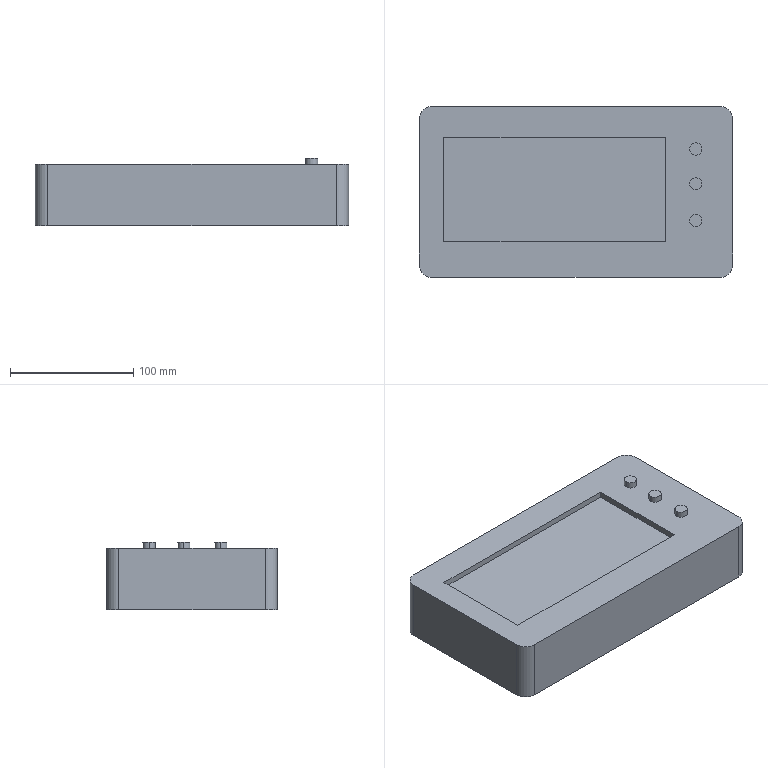Part | STEP file | Controller | 1 solid | 27 faces | box 254.791 x 138.794 x 55 mm | volume 1688527 mm3 | plane 15 | cylinder 12 | commonest cylinder face diameters 10 x6 20 x4 2 x2
STEP:
#1=CARTESIAN_POINT('',(-10.,-56.504,29.99));
#2=VERTEX_POINT('',#1);
#3=CARTESIAN_POINT('',(-10.,-56.504,27.99));
#4=VERTEX_POINT('',#3);
#5=CARTESIAN_POINT('',(-10.,-56.504,28.99));
#6=DIRECTION('',(1.,0.,0.));
#7=DIRECTION('',(0.,0.,-1.));
#8=AXIS2_PLACEMENT_3D('',#5,#6,#7);
#9=CIRCLE('',#8,1.);
#10=EDGE_CURVE('',#2,#4,#9,.T.);
#11=ORIENTED_EDGE('',*,*,#10,.F.);
#12=CARTESIAN_POINT('',(0.,-56.504,29.99));
#13=VERTEX_POINT('',#12);
#14=CARTESIAN_POINT('',(-10.,-56.504,29.99));
#15=DIRECTION('',(1.,0.,0.));
#16=VECTOR('',#15,1000.);
#17=LINE('',#14,#16);
#18=EDGE_CURVE('',#2,#13,#17,.T.);
#19=ORIENTED_EDGE('',*,*,#18,.T.);
#20=CARTESIAN_POINT('',(0.,-56.504,27.99));
#21=VERTEX_POINT('',#20);
#22=CARTESIAN_POINT('',(0.,-56.504,28.99));
#23=DIRECTION('',(1.,0.,0.));
#24=DIRECTION('',(0.,0.,-1.));
#25=AXIS2_PLACEMENT_3D('',#22,#23,#24);
#26=CIRCLE('',#25,1.);
#27=EDGE_CURVE('',#13,#21,#26,.T.);
#28=ORIENTED_EDGE('',*,*,#27,.T.);
#29=CARTESIAN_POINT('',(-10.,-56.504,27.99));
#30=DIRECTION('',(1.,0.,0.));
#31=VECTOR('',#30,1000.);
#32=LINE('',#29,#31);
#33=EDGE_CURVE('',#4,#21,#32,.T.);
#34=ORIENTED_EDGE('',*,*,#33,.F.);
#35=EDGE_LOOP('',(#11,#19,#28,#34));
#36=FACE_OUTER_BOUND('',#35,.T.);
#37=CARTESIAN_POINT('',(-10.,-56.504,28.99));
#38=DIRECTION('',(1.,0.,0.));
#39=DIRECTION('',(0.,0.,-1.));
#40=AXIS2_PLACEMENT_3D('',#37,#38,#39);
#41=CYLINDRICAL_SURFACE('',#40,1.);
#42=ADVANCED_FACE('',(#36),#41,.F.);
#43=CARTESIAN_POINT('',(-25.,-92.807,55.));
#44=VERTEX_POINT('',#43);
#45=CARTESIAN_POINT('',(-35.,-92.807,55.));
#46=VERTEX_POINT('',#45);
#47=CARTESIAN_POINT('',(-30.,-92.807,55.));
#48=DIRECTION('',(0.,0.,1.));
#49=DIRECTION('',(1.,0.,0.));
#50=AXIS2_PLACEMENT_3D('',#47,#48,#49);
#51=CIRCLE('',#50,5.);
#52=EDGE_CURVE('',#44,#46,#51,.T.);
#53=ORIENTED_EDGE('',*,*,#52,.F.);
#54=CARTESIAN_POINT('',(-25.,-92.807,50.));
#55=VERTEX_POINT('',#54);
#56=CARTESIAN_POINT('',(-25.,-92.807,55.));
#57=DIRECTION('',(0.,0.,-1.));
#58=VECTOR('',#57,1000.);
#59=LINE('',#56,#58);
#60=EDGE_CURVE('',#44,#55,#59,.T.);
#61=ORIENTED_EDGE('',*,*,#60,.T.);
#62=CARTESIAN_POINT('',(-35.,-92.807,50.));
#63=VERTEX_POINT('',#62);
#64=CARTESIAN_POINT('',(-30.,-92.807,50.));
#65=DIRECTION('',(0.,0.,1.));
#66=DIRECTION('',(1.,0.,0.));
#67=AXIS2_PLACEMENT_3D('',#64,#65,#66);
#68=CIRCLE('',#67,5.);
#69=EDGE_CURVE('',#55,#63,#68,.T.);
#70=ORIENTED_EDGE('',*,*,#69,.T.);
#71=CARTESIAN_POINT('',(-35.,-92.807,55.));
#72=DIRECTION('',(0.,0.,-1.));
#73=VECTOR('',#72,1000.);
#74=LINE('',#71,#73);
#75=EDGE_CURVE('',#46,#63,#74,.T.);
#76=ORIENTED_EDGE('',*,*,#75,.F.);
#77=EDGE_LOOP('',(#53,#61,#70,#76));
#78=FACE_OUTER_BOUND('',#77,.T.);
#79=CARTESIAN_POINT('',(-30.,-92.807,55.));
#80=DIRECTION('',(0.,0.,-1.));
#81=DIRECTION('',(-1.,0.,0.));
#82=AXIS2_PLACEMENT_3D('',#79,#80,#81);
#83=CYLINDRICAL_SURFACE('',#82,5.);
#84=ADVANCED_FACE('',(#78),#83,.T.);
#85=CARTESIAN_POINT('',(-25.,-62.807,55.));
#86=VERTEX_POINT('',#85);
#87=CARTESIAN_POINT('',(-35.,-62.807,55.));
#88=VERTEX_POINT('',#87);
#89=CARTESIAN_POINT('',(-30.,-62.807,55.));
#90=DIRECTION('',(0.,0.,1.));
#91=DIRECTION('',(1.,0.,0.));
#92=AXIS2_PLACEMENT_3D('',#89,#90,#91);
#93=CIRCLE('',#92,5.);
#94=EDGE_CURVE('',#86,#88,#93,.T.);
#95=ORIENTED_EDGE('',*,*,#94,.F.);
#96=CARTESIAN_POINT('',(-25.,-62.807,50.));
#97=VERTEX_POINT('',#96);
#98=CARTESIAN_POINT('',(-25.,-62.807,55.));
#99=DIRECTION('',(0.,0.,-1.));
#100=VECTOR('',#99,1000.);
#101=LINE('',#98,#100);
#102=EDGE_CURVE('',#86,#97,#101,.T.);
#103=ORIENTED_EDGE('',*,*,#102,.T.);
#104=CARTESIAN_POINT('',(-35.,-62.807,50.));
#105=VERTEX_POINT('',#104);
#106=CARTESIAN_POINT('',(-30.,-62.807,50.));
#107=DIRECTION('',(0.,0.,1.));
#108=DIRECTION('',(1.,0.,0.));
#109=AXIS2_PLACEMENT_3D('',#106,#107,#108);
#110=CIRCLE('',#109,5.);
#111=EDGE_CURVE('',#97,#105,#110,.T.);
#112=ORIENTED_EDGE('',*,*,#111,.T.);
#113=CARTESIAN_POINT('',(-35.,-62.807,55.));
#114=DIRECTION('',(0.,0.,-1.));
#115=VECTOR('',#114,1000.);
#116=LINE('',#113,#115);
#117=EDGE_CURVE('',#88,#105,#116,.T.);
#118=ORIENTED_EDGE('',*,*,#117,.F.);
#119=EDGE_LOOP('',(#95,#103,#112,#118));
#120=FACE_OUTER_BOUND('',#119,.T.);
#121=CARTESIAN_POINT('',(-30.,-62.807,55.));
#122=DIRECTION('',(0.,0.,-1.));
#123=DIRECTION('',(-1.,0.,0.));
#124=AXIS2_PLACEMENT_3D('',#121,#122,#123);
#125=CYLINDRICAL_SURFACE('',#124,5.);
#126=ADVANCED_FACE('',(#120),#125,.T.);
#127=CARTESIAN_POINT('',(-25.,-34.514,55.));
#128=VERTEX_POINT('',#127);
#129=CARTESIAN_POINT('',(-35.,-34.514,55.));
#130=VERTEX_POINT('',#129);
#131=CARTESIAN_POINT('',(-30.,-34.514,55.));
#132=DIRECTION('',(0.,0.,1.));
#133=DIRECTION('',(1.,0.,0.));
#134=AXIS2_PLACEMENT_3D('',#131,#132,#133);
#135=CIRCLE('',#134,5.);
#136=EDGE_CURVE('',#128,#130,#135,.T.);
#137=ORIENTED_EDGE('',*,*,#136,.F.);
#138=CARTESIAN_POINT('',(-25.,-34.514,50.));
#139=VERTEX_POINT('',#138);
#140=CARTESIAN_POINT('',(-25.,-34.514,55.));
#141=DIRECTION('',(0.,0.,-1.));
#142=VECTOR('',#141,1000.);
#143=LINE('',#140,#142);
#144=EDGE_CURVE('',#128,#139,#143,.T.);
#145=ORIENTED_EDGE('',*,*,#144,.T.);
#146=CARTESIAN_POINT('',(-35.,-34.514,50.));
#147=VERTEX_POINT('',#146);
#148=CARTESIAN_POINT('',(-30.,-34.514,50.));
#149=DIRECTION('',(0.,0.,1.));
#150=DIRECTION('',(1.,0.,0.));
#151=AXIS2_PLACEMENT_3D('',#148,#149,#150);
#152=CIRCLE('',#151,5.);
#153=EDGE_CURVE('',#139,#147,#152,.T.);
#154=ORIENTED_EDGE('',*,*,#153,.T.);
#155=CARTESIAN_POINT('',(-35.,-34.514,55.));
#156=DIRECTION('',(0.,0.,-1.));
#157=VECTOR('',#156,1000.);
#158=LINE('',#155,#157);
#159=EDGE_CURVE('',#130,#147,#158,.T.);
#160=ORIENTED_EDGE('',*,*,#159,.F.);
#161=EDGE_LOOP('',(#137,#145,#154,#160));
#162=FACE_OUTER_BOUND('',#161,.T.);
#163=CARTESIAN_POINT('',(-30.,-34.514,55.));
#164=DIRECTION('',(0.,0.,-1.));
#165=DIRECTION('',(-1.,0.,0.));
#166=AXIS2_PLACEMENT_3D('',#163,#164,#165);
#167=CYLINDRICAL_SURFACE('',#166,5.);
#168=ADVANCED_FACE('',(#162),#167,.T.);
#169=CARTESIAN_POINT('',(-254.791,-128.794,0.));
#170=VERTEX_POINT('',#169);
#171=CARTESIAN_POINT('',(-244.791,-138.794,0.));
#172=VERTEX_POINT('',#171);
#173=CARTESIAN_POINT('',(-244.791,-128.794,0.));
#174=DIRECTION('',(0.,0.,1.));
#175=DIRECTION('',(1.,0.,0.));
#176=AXIS2_PLACEMENT_3D('',#173,#174,#175);
#177=CIRCLE('',#176,10.);
#178=EDGE_CURVE('',#170,#172,#177,.T.);
#179=ORIENTED_EDGE('',*,*,#178,.T.);
#180=CARTESIAN_POINT('',(-244.791,-138.794,50.));
#181=VERTEX_POINT('',#180);
#182=CARTESIAN_POINT('',(-244.791,-138.794,50.));
#183=DIRECTION('',(0.,0.,-1.));
#184=VECTOR('',#183,1000.);
#185=LINE('',#182,#184);
#186=EDGE_CURVE('',#181,#172,#185,.T.);
#187=ORIENTED_EDGE('',*,*,#186,.F.);
#188=CARTESIAN_POINT('',(-254.791,-128.794,50.));
#189=VERTEX_POINT('',#188);
#190=CARTESIAN_POINT('',(-244.791,-128.794,50.));
#191=DIRECTION('',(0.,0.,1.));
#192=DIRECTION('',(1.,0.,0.));
#193=AXIS2_PLACEMENT_3D('',#190,#191,#192);
#194=CIRCLE('',#193,10.);
#195=EDGE_CURVE('',#189,#181,#194,.T.);
#196=ORIENTED_EDGE('',*,*,#195,.F.);
#197=CARTESIAN_POINT('',(-254.791,-128.794,50.));
#198=DIRECTION('',(0.,0.,-1.));
#199=VECTOR('',#198,1000.);
#200=LINE('',#197,#199);
#201=EDGE_CURVE('',#189,#170,#200,.T.);
#202=ORIENTED_EDGE('',*,*,#201,.T.);
#203=EDGE_LOOP('',(#179,#187,#196,#202));
#204=FACE_OUTER_BOUND('',#203,.T.);
#205=CARTESIAN_POINT('',(-244.791,-128.794,50.));
#206=DIRECTION('',(0.,0.,-1.));
#207=DIRECTION('',(-1.,0.,0.));
#208=AXIS2_PLACEMENT_3D('',#205,#206,#207);
#209=CYLINDRICAL_SURFACE('',#208,10.);
#210=ADVANCED_FACE('',(#204),#209,.T.);
#211=CARTESIAN_POINT('',(-10.,-138.794,0.));
#212=VERTEX_POINT('',#211);
#213=CARTESIAN_POINT('',(-244.791,-138.794,0.));
#214=DIRECTION('',(1.,0.,0.));
#215=VECTOR('',#214,1000.);
#216=LINE('',#213,#215);
#217=EDGE_CURVE('',#172,#212,#216,.T.);
#218=ORIENTED_EDGE('',*,*,#217,.T.);
#219=CARTESIAN_POINT('',(-10.,-138.794,50.));
#220=VERTEX_POINT('',#219);
#221=CARTESIAN_POINT('',(-10.,-138.794,50.));
#222=DIRECTION('',(0.,0.,-1.));
#223=VECTOR('',#222,1000.);
#224=LINE('',#221,#223);
#225=EDGE_CURVE('',#220,#212,#224,.T.);
#226=ORIENTED_EDGE('',*,*,#225,.F.);
#227=CARTESIAN_POINT('',(-244.791,-138.794,50.));
#228=DIRECTION('',(1.,0.,0.));
#229=VECTOR('',#228,1000.);
#230=LINE('',#227,#229);
#231=EDGE_CURVE('',#181,#220,#230,.T.);
#232=ORIENTED_EDGE('',*,*,#231,.F.);
#233=ORIENTED_EDGE('',*,*,#186,.T.);
#234=EDGE_LOOP('',(#218,#226,#232,#233));
#235=FACE_OUTER_BOUND('',#234,.T.);
#236=CARTESIAN_POINT('',(-244.791,-138.794,50.));
#237=DIRECTION('',(0.,1.,0.));
#238=DIRECTION('',(0.,0.,1.));
#239=AXIS2_PLACEMENT_3D('',#236,#237,#238);
#240=PLANE('',#239);
#241=ADVANCED_FACE('',(#235),#240,.F.);
#242=CARTESIAN_POINT('',(0.,-128.794,0.));
#243=VERTEX_POINT('',#242);
#244=CARTESIAN_POINT('',(-10.,-128.794,0.));
#245=DIRECTION('',(0.,0.,1.));
#246=DIRECTION('',(1.,0.,0.));
#247=AXIS2_PLACEMENT_3D('',#244,#245,#246);
#248=CIRCLE('',#247,10.);
#249=EDGE_CURVE('',#212,#243,#248,.T.);
#250=ORIENTED_EDGE('',*,*,#249,.T.);
#251=CARTESIAN_POINT('',(0.,-128.794,50.));
#252=VERTEX_POINT('',#251);
#253=CARTESIAN_POINT('',(0.,-128.794,50.));
#254=DIRECTION('',(0.,0.,-1.));
#255=VECTOR('',#254,1000.);
#256=LINE('',#253,#255);
#257=EDGE_CURVE('',#252,#243,#256,.T.);
#258=ORIENTED_EDGE('',*,*,#257,.F.);
#259=CARTESIAN_POINT('',(-10.,-128.794,50.));
#260=DIRECTION('',(0.,0.,1.));
#261=DIRECTION('',(1.,0.,0.));
#262=AXIS2_PLACEMENT_3D('',#259,#260,#261);
#263=CIRCLE('',#262,10.);
#264=EDGE_CURVE('',#220,#252,#263,.T.);
#265=ORIENTED_EDGE('',*,*,#264,.F.);
#266=ORIENTED_EDGE('',*,*,#225,.T.);
#267=EDGE_LOOP('',(#250,#258,#265,#266));
#268=FACE_OUTER_BOUND('',#267,.T.);
#269=CARTESIAN_POINT('',(-10.,-128.794,50.));
#270=DIRECTION('',(0.,0.,-1.));
#271=DIRECTION('',(-1.,0.,0.));
#272=AXIS2_PLACEMENT_3D('',#269,#270,#271);
#273=CYLINDRICAL_SURFACE('',#272,10.);
#274=ADVANCED_FACE('',(#268),#273,.T.);
#275=CARTESIAN_POINT('',(0.,-56.504,28.99));
#276=DIRECTION('',(1.,0.,0.));
#277=DIRECTION('',(0.,0.,-1.));
#278=AXIS2_PLACEMENT_3D('',#275,#276,#277);
#279=CIRCLE('',#278,1.);
#280=EDGE_CURVE('',#21,#13,#279,.T.);
#281=ORIENTED_EDGE('',*,*,#280,.F.);
#282=ORIENTED_EDGE('',*,*,#27,.F.);
#283=EDGE_LOOP('',(#281,#282));
#284=FACE_BOUND('',#283,.T.);
#285=CARTESIAN_POINT('',(0.,-10.,0.));
#286=VERTEX_POINT('',#285);
#287=CARTESIAN_POINT('',(0.,-128.794,0.));
#288=DIRECTION('',(0.,1.,0.));
#289=VECTOR('',#288,1000.);
#290=LINE('',#287,#289);
#291=EDGE_CURVE('',#243,#286,#290,.T.);
#292=ORIENTED_EDGE('',*,*,#291,.T.);
#293=CARTESIAN_POINT('',(0.,-10.,50.));
#294=VERTEX_POINT('',#293);
#295=CARTESIAN_POINT('',(0.,-10.,50.));
#296=DIRECTION('',(0.,0.,-1.));
#297=VECTOR('',#296,1000.);
#298=LINE('',#295,#297);
#299=EDGE_CURVE('',#294,#286,#298,.T.);
#300=ORIENTED_EDGE('',*,*,#299,.F.);
#301=CARTESIAN_POINT('',(0.,-128.794,50.));
#302=DIRECTION('',(0.,1.,0.));
#303=VECTOR('',#302,1000.);
#304=LINE('',#301,#303);
#305=EDGE_CURVE('',#252,#294,#304,.T.);
#306=ORIENTED_EDGE('',*,*,#305,.F.);
#307=ORIENTED_EDGE('',*,*,#257,.T.);
#308=EDGE_LOOP('',(#292,#300,#306,#307));
#309=FACE_OUTER_BOUND('',#308,.T.);
#310=CARTESIAN_POINT('',(0.,-128.794,50.));
#311=DIRECTION('',(-1.,0.,0.));
#312=DIRECTION('',(0.,0.,1.));
#313=AXIS2_PLACEMENT_3D('',#310,#311,#312);
#314=PLANE('',#313);
#315=ADVANCED_FACE('',(#284,#309),#314,.F.);
#316=CARTESIAN_POINT('',(-10.,0.,0.));
#317=VERTEX_POINT('',#316);
#318=CARTESIAN_POINT('',(-10.,-10.,0.));
#319=DIRECTION('',(0.,0.,1.));
#320=DIRECTION('',(1.,0.,0.));
#321=AXIS2_PLACEMENT_3D('',#318,#319,#320);
#322=CIRCLE('',#321,10.);
#323=EDGE_CURVE('',#286,#317,#322,.T.);
#324=ORIENTED_EDGE('',*,*,#323,.T.);
#325=CARTESIAN_POINT('',(-10.,0.,50.));
#326=VERTEX_POINT('',#325);
#327=CARTESIAN_POINT('',(-10.,0.,50.));
#328=DIRECTION('',(0.,0.,-1.));
#329=VECTOR('',#328,1000.);
#330=LINE('',#327,#329);
#331=EDGE_CURVE('',#326,#317,#330,.T.);
#332=ORIENTED_EDGE('',*,*,#331,.F.);
#333=CARTESIAN_POINT('',(-10.,-10.,50.));
#334=DIRECTION('',(0.,0.,1.));
#335=DIRECTION('',(1.,0.,0.));
#336=AXIS2_PLACEMENT_3D('',#333,#334,#335);
#337=CIRCLE('',#336,10.);
#338=EDGE_CURVE('',#294,#326,#337,.T.);
#339=ORIENTED_EDGE('',*,*,#338,.F.);
#340=ORIENTED_EDGE('',*,*,#299,.T.);
#341=EDGE_LOOP('',(#324,#332,#339,#340));
#342=FACE_OUTER_BOUND('',#341,.T.);
#343=CARTESIAN_POINT('',(-10.,-10.,50.));
#344=DIRECTION('',(0.,0.,-1.));
#345=DIRECTION('',(-1.,0.,0.));
#346=AXIS2_PLACEMENT_3D('',#343,#344,#345);
#347=CYLINDRICAL_SURFACE('',#346,10.);
#348=ADVANCED_FACE('',(#342),#347,.T.);
#349=CARTESIAN_POINT('',(-244.791,0.,0.));
#350=VERTEX_POINT('',#349);
#351=CARTESIAN_POINT('',(-10.,0.,0.));
#352=DIRECTION('',(-1.,0.,0.));
#353=VECTOR('',#352,1000.);
#354=LINE('',#351,#353);
#355=EDGE_CURVE('',#317,#350,#354,.T.);
#356=ORIENTED_EDGE('',*,*,#355,.T.);
#357=CARTESIAN_POINT('',(-244.791,0.,50.));
#358=VERTEX_POINT('',#357);
#359=CARTESIAN_POINT('',(-244.791,0.,50.));
#360=DIRECTION('',(0.,0.,-1.));
#361=VECTOR('',#360,1000.);
#362=LINE('',#359,#361);
#363=EDGE_CURVE('',#358,#350,#362,.T.);
#364=ORIENTED_EDGE('',*,*,#363,.F.);
#365=CARTESIAN_POINT('',(-10.,0.,50.));
#366=DIRECTION('',(-1.,0.,0.));
#367=VECTOR('',#366,1000.);
#368=LINE('',#365,#367);
#369=EDGE_CURVE('',#326,#358,#368,.T.);
#370=ORIENTED_EDGE('',*,*,#369,.F.);
#371=ORIENTED_EDGE('',*,*,#331,.T.);
#372=EDGE_LOOP('',(#356,#364,#370,#371));
#373=FACE_OUTER_BOUND('',#372,.T.);
#374=CARTESIAN_POINT('',(-10.,0.,50.));
#375=DIRECTION('',(0.,-1.,0.));
#376=DIRECTION('',(1.,0.,0.));
#377=AXIS2_PLACEMENT_3D('',#374,#375,#376);
#378=PLANE('',#377);
#379=ADVANCED_FACE('',(#373),#378,.F.);
#380=CARTESIAN_POINT('',(-254.791,-10.,0.));
#381=VERTEX_POINT('',#380);
#382=CARTESIAN_POINT('',(-244.791,-10.,0.));
#383=DIRECTION('',(0.,0.,1.));
#384=DIRECTION('',(1.,0.,0.));
#385=AXIS2_PLACEMENT_3D('',#382,#383,#384);
#386=CIRCLE('',#385,10.);
#387=EDGE_CURVE('',#350,#381,#386,.T.);
#388=ORIENTED_EDGE('',*,*,#387,.T.);
#389=CARTESIAN_POINT('',(-254.791,-10.,50.));
#390=VERTEX_POINT('',#389);
#391=CARTESIAN_POINT('',(-254.791,-10.,50.));
#392=DIRECTION('',(0.,0.,-1.));
#393=VECTOR('',#392,1000.);
#394=LINE('',#391,#393);
#395=EDGE_CURVE('',#390,#381,#394,.T.);
#396=ORIENTED_EDGE('',*,*,#395,.F.);
#397=CARTESIAN_POINT('',(-244.791,-10.,50.));
#398=DIRECTION('',(0.,0.,1.));
#399=DIRECTION('',(1.,0.,0.));
#400=AXIS2_PLACEMENT_3D('',#397,#398,#399);
#401=CIRCLE('',#400,10.);
#402=EDGE_CURVE('',#358,#390,#401,.T.);
#403=ORIENTED_EDGE('',*,*,#402,.F.);
#404=ORIENTED_EDGE('',*,*,#363,.T.);
#405=EDGE_LOOP('',(#388,#396,#403,#404));
#406=FACE_OUTER_BOUND('',#405,.T.);
#407=CARTESIAN_POINT('',(-244.791,-10.,50.));
#408=DIRECTION('',(0.,0.,-1.));
#409=DIRECTION('',(-1.,0.,0.));
#410=AXIS2_PLACEMENT_3D('',#407,#408,#409);
#411=CYLINDRICAL_SURFACE('',#410,10.);
#412=ADVANCED_FACE('',(#406),#411,.T.);
#413=CARTESIAN_POINT('',(-254.791,-10.,0.));
#414=DIRECTION('',(0.,-1.,0.));
#415=VECTOR('',#414,1000.);
#416=LINE('',#413,#415);
#417=EDGE_CURVE('',#381,#170,#416,.T.);
#418=ORIENTED_EDGE('',*,*,#417,.T.);
#419=ORIENTED_EDGE('',*,*,#201,.F.);
#420=CARTESIAN_POINT('',(-254.791,-10.,50.));
#421=DIRECTION('',(0.,-1.,0.));
#422=VECTOR('',#421,1000.);
#423=LINE('',#420,#422);
#424=EDGE_CURVE('',#390,#189,#423,.T.);
#425=ORIENTED_EDGE('',*,*,#424,.F.);
#426=ORIENTED_EDGE('',*,*,#395,.T.);
#427=EDGE_LOOP('',(#418,#419,#425,#426));
#428=FACE_OUTER_BOUND('',#427,.T.);
#429=CARTESIAN_POINT('',(-254.791,-10.,50.));
#430=DIRECTION('',(1.,0.,0.));
#431=DIRECTION('',(0.,0.,-1.));
#432=AXIS2_PLACEMENT_3D('',#429,#430,#431);
#433=PLANE('',#432);
#434=ADVANCED_FACE('',(#428),#433,.F.);
#435=CARTESIAN_POINT('',(-30.,-92.807,50.));
#436=DIRECTION('',(0.,0.,1.));
#437=DIRECTION('',(1.,0.,0.));
#438=AXIS2_PLACEMENT_3D('',#435,#436,#437);
#439=CIRCLE('',#438,5.);
#440=EDGE_CURVE('',#63,#55,#439,.T.);
#441=ORIENTED_EDGE('',*,*,#440,.F.);
#442=ORIENTED_EDGE('',*,*,#69,.F.);
#443=EDGE_LOOP('',(#441,#442));
#444=FACE_BOUND('',#443,.T.);
#445=CARTESIAN_POINT('',(-30.,-62.807,50.));
#446=DIRECTION('',(0.,0.,1.));
#447=DIRECTION('',(1.,0.,0.));
#448=AXIS2_PLACEMENT_3D('',#445,#446,#447);
#449=CIRCLE('',#448,5.);
#450=EDGE_CURVE('',#105,#97,#449,.T.);
#451=ORIENTED_EDGE('',*,*,#450,.F.);
#452=ORIENTED_EDGE('',*,*,#111,.F.);
#453=EDGE_LOOP('',(#451,#452));
#454=FACE_BOUND('',#453,.T.);
#455=CARTESIAN_POINT('',(-30.,-34.514,50.));
#456=DIRECTION('',(0.,0.,1.));
#457=DIRECTION('',(1.,0.,0.));
#458=AXIS2_PLACEMENT_3D('',#455,#456,#457);
#459=CIRCLE('',#458,5.);
#460=EDGE_CURVE('',#147,#139,#459,.T.);
#461=ORIENTED_EDGE('',*,*,#460,.F.);
#462=ORIENTED_EDGE('',*,*,#153,.F.);
#463=EDGE_LOOP('',(#461,#462));
#464=FACE_BOUND('',#463,.T.);
#465=CARTESIAN_POINT('',(-234.791,-110.,50.));
#466=VERTEX_POINT('',#465);
#467=CARTESIAN_POINT('',(-54.791,-110.,50.));
#468=VERTEX_POINT('',#467);
#469=CARTESIAN_POINT('',(-234.791,-110.,50.));
#470=DIRECTION('',(1.,0.,0.));
#471=VECTOR('',#470,1000.);
#472=LINE('',#469,#471);
#473=EDGE_CURVE('',#466,#468,#472,.T.);
#474=ORIENTED_EDGE('',*,*,#473,.F.);
#475=CARTESIAN_POINT('',(-234.791,-25.,50.));
#476=VERTEX_POINT('',#475);
#477=CARTESIAN_POINT('',(-234.791,-25.,50.));
#478=DIRECTION('',(0.,-1.,0.));
#479=VECTOR('',#478,1000.);
#480=LINE('',#477,#479);
#481=EDGE_CURVE('',#476,#466,#480,.T.);
#482=ORIENTED_EDGE('',*,*,#481,.F.);
#483=CARTESIAN_POINT('',(-54.791,-25.,50.));
#484=VERTEX_POINT('',#483);
#485=CARTESIAN_POINT('',(-234.791,-25.,50.));
#486=DIRECTION('',(-1.,0.,0.));
#487=VECTOR('',#486,1000.);
#488=LINE('',#485,#487);
#489=EDGE_CURVE('',#484,#476,#488,.T.);
#490=ORIENTED_EDGE('',*,*,#489,.F.);
#491=CARTESIAN_POINT('',(-54.791,-110.,50.));
#492=DIRECTION('',(0.,1.,0.));
#493=VECTOR('',#492,1000.);
#494=LINE('',#491,#493);
#495=EDGE_CURVE('',#468,#484,#494,.T.);
#496=ORIENTED_EDGE('',*,*,#495,.F.);
#497=EDGE_LOOP('',(#474,#482,#490,#496));
#498=FACE_BOUND('',#497,.T.);
#499=ORIENTED_EDGE('',*,*,#195,.T.);
#500=ORIENTED_EDGE('',*,*,#231,.T.);
#501=ORIENTED_EDGE('',*,*,#264,.T.);
#502=ORIENTED_EDGE('',*,*,#305,.T.);
#503=ORIENTED_EDGE('',*,*,#338,.T.);
#504=ORIENTED_EDGE('',*,*,#369,.T.);
#505=ORIENTED_EDGE('',*,*,#402,.T.);
#506=ORIENTED_EDGE('',*,*,#424,.T.);
#507=EDGE_LOOP('',(#499,#500,#501,#502,#503,#504,#505,#506));
#508=FACE_OUTER_BOUND('',#507,.T.);
#509=CARTESIAN_POINT('',(-244.791,-128.794,50.));
#510=DIRECTION('',(0.,0.,1.));
#511=DIRECTION('',(1.,0.,0.));
#512=AXIS2_PLACEMENT_3D('',#509,#510,#511);
#513=PLANE('',#512);
#514=ADVANCED_FACE('',(#444,#454,#464,#498,#508),#513,.T.);
#515=ORIENTED_EDGE('',*,*,#178,.F.);
#516=ORIENTED_EDGE('',*,*,#417,.F.);
#517=ORIENTED_EDGE('',*,*,#387,.F.);
#518=ORIENTED_EDGE('',*,*,#355,.F.);
#519=ORIENTED_EDGE('',*,*,#323,.F.);
#520=ORIENTED_EDGE('',*,*,#291,.F.);
#521=ORIENTED_EDGE('',*,*,#249,.F.);
#522=ORIENTED_EDGE('',*,*,#217,.F.);
#523=EDGE_LOOP('',(#515,#516,#517,#518,#519,#520,#521,#522));
#524=FACE_OUTER_BOUND('',#523,.T.);
#525=CARTESIAN_POINT('',(-244.791,-128.794,0.));
#526=DIRECTION('',(0.,0.,1.));
#527=DIRECTION('',(1.,0.,0.));
#528=AXIS2_PLACEMENT_3D('',#525,#526,#527);
#529=PLANE('',#528);
#530=ADVANCED_FACE('',(#524),#529,.F.);
#531=ORIENTED_EDGE('',*,*,#473,.T.);
#532=CARTESIAN_POINT('',(-54.791,-110.,45.));
#533=VERTEX_POINT('',#532);
#534=CARTESIAN_POINT('',(-54.791,-110.,45.));
#535=DIRECTION('',(0.,0.,1.));
#536=VECTOR('',#535,1000.);
#537=LINE('',#534,#536);
#538=EDGE_CURVE('',#533,#468,#537,.T.);
#539=ORIENTED_EDGE('',*,*,#538,.F.);
#540=CARTESIAN_POINT('',(-234.791,-110.,45.));
#541=VERTEX_POINT('',#540);
#542=CARTESIAN_POINT('',(-234.791,-110.,45.));
#543=DIRECTION('',(1.,0.,0.));
#544=VECTOR('',#543,1000.);
#545=LINE('',#542,#544);
#546=EDGE_CURVE('',#541,#533,#545,.T.);
#547=ORIENTED_EDGE('',*,*,#546,.F.);
#548=CARTESIAN_POINT('',(-234.791,-110.,45.));
#549=DIRECTION('',(0.,0.,1.));
#550=VECTOR('',#549,1000.);
#551=LINE('',#548,#550);
#552=EDGE_CURVE('',#541,#466,#551,.T.);
#553=ORIENTED_EDGE('',*,*,#552,.T.);
#554=EDGE_LOOP('',(#531,#539,#547,#553));
#555=FACE_OUTER_BOUND('',#554,.T.);
#556=CARTESIAN_POINT('',(-234.791,-110.,45.));
#557=DIRECTION('',(0.,-1.,0.));
#558=DIRECTION('',(0.,0.,-1.));
#559=AXIS2_PLACEMENT_3D('',#556,#557,#558);
#560=PLANE('',#559);
#561=ADVANCED_FACE('',(#555),#560,.F.);
#562=ORIENTED_EDGE('',*,*,#481,.T.);
#563=ORIENTED_EDGE('',*,*,#552,.F.);
#564=CARTESIAN_POINT('',(-234.791,-25.,45.));
#565=VERTEX_POINT('',#564);
#566=CARTESIAN_POINT('',(-234.791,-25.,45.));
#567=DIRECTION('',(0.,-1.,0.));
#568=VECTOR('',#567,1000.);
#569=LINE('',#566,#568);
#570=EDGE_CURVE('',#565,#541,#569,.T.);
#571=ORIENTED_EDGE('',*,*,#570,.F.);
#572=CARTESIAN_POINT('',(-234.791,-25.,45.));
#573=DIRECTION('',(0.,0.,1.));
#574=VECTOR('',#573,1000.);
#575=LINE('',#572,#574);
#576=EDGE_CURVE('',#565,#476,#575,.T.);
#577=ORIENTED_EDGE('',*,*,#576,.T.);
#578=EDGE_LOOP('',(#562,#563,#571,#577));
#579=FACE_OUTER_BOUND('',#578,.T.);
#580=CARTESIAN_POINT('',(-234.791,-25.,45.));
#581=DIRECTION('',(-1.,0.,0.));
#582=DIRECTION('',(0.,0.,1.));
#583=AXIS2_PLACEMENT_3D('',#580,#581,#582);
#584=PLANE('',#583);
#585=ADVANCED_FACE('',(#579),#584,.F.);
#586=ORIENTED_EDGE('',*,*,#489,.T.);
#587=ORIENTED_EDGE('',*,*,#576,.F.);
#588=CARTESIAN_POINT('',(-54.791,-25.,45.));
#589=VERTEX_POINT('',#588);
#590=CARTESIAN_POINT('',(-234.791,-25.,45.));
#591=DIRECTION('',(-1.,0.,0.));
#592=VECTOR('',#591,1000.);
#593=LINE('',#590,#592);
#594=EDGE_CURVE('',#589,#565,#593,.T.);
#595=ORIENTED_EDGE('',*,*,#594,.F.);
#596=CARTESIAN_POINT('',(-54.791,-25.,45.));
#597=DIRECTION('',(0.,0.,1.));
#598=VECTOR('',#597,1000.);
#599=LINE('',#596,#598);
#600=EDGE_CURVE('',#589,#484,#599,.T.);
#601=ORIENTED_EDGE('',*,*,#600,.T.);
#602=EDGE_LOOP('',(#586,#587,#595,#601));
#603=FACE_OUTER_BOUND('',#602,.T.);
#604=CARTESIAN_POINT('',(-234.791,-25.,45.));
#605=DIRECTION('',(0.,1.,0.));
#606=DIRECTION('',(0.,0.,1.));
#607=AXIS2_PLACEMENT_3D('',#604,#605,#606);
#608=PLANE('',#607);
#609=ADVANCED_FACE('',(#603),#608,.F.);
#610=ORIENTED_EDGE('',*,*,#495,.T.);
#611=ORIENTED_EDGE('',*,*,#600,.F.);
#612=CARTESIAN_POINT('',(-54.791,-110.,45.));
#613=DIRECTION('',(0.,1.,0.));
#614=VECTOR('',#613,1000.);
#615=LINE('',#612,#614);
#616=EDGE_CURVE('',#533,#589,#615,.T.);
#617=ORIENTED_EDGE('',*,*,#616,.F.);
#618=ORIENTED_EDGE('',*,*,#538,.T.);
#619=EDGE_LOOP('',(#610,#611,#617,#618));
#620=FACE_OUTER_BOUND('',#619,.T.);
#621=CARTESIAN_POINT('',(-54.791,-110.,45.));
#622=DIRECTION('',(1.,0.,0.));
#623=DIRECTION('',(0.,0.,-1.));
#624=AXIS2_PLACEMENT_3D('',#621,#622,#623);
#625=PLANE('',#624);
#626=ADVANCED_FACE('',(#620),#625,.F.);
#627=ORIENTED_EDGE('',*,*,#546,.T.);
#628=ORIENTED_EDGE('',*,*,#616,.T.);
#629=ORIENTED_EDGE('',*,*,#594,.T.);
#630=ORIENTED_EDGE('',*,*,#570,.T.);
#631=EDGE_LOOP('',(#627,#628,#629,#630));
#632=FACE_OUTER_BOUND('',#631,.T.);
#633=CARTESIAN_POINT('',(0.,0.,45.));
#634=DIRECTION('',(0.,0.,1.));
#635=DIRECTION('',(1.,0.,0.));
#636=AXIS2_PLACEMENT_3D('',#633,#634,#635);
#637=PLANE('',#636);
#638=ADVANCED_FACE('',(#632),#637,.T.);
#639=ORIENTED_EDGE('',*,*,#144,.F.);
#640=CARTESIAN_POINT('',(-30.,-34.514,55.));
#641=DIRECTION('',(0.,0.,1.));
#642=DIRECTION('',(1.,0.,0.));
#643=AXIS2_PLACEMENT_3D('',#640,#641,#642);
#644=CIRCLE('',#643,5.);
#645=EDGE_CURVE('',#130,#128,#644,.T.);
#646=ORIENTED_EDGE('',*,*,#645,.F.);
#647=ORIENTED_EDGE('',*,*,#159,.T.);
#648=ORIENTED_EDGE('',*,*,#460,.T.);
#649=EDGE_LOOP('',(#639,#646,#647,#648));
#650=FACE_OUTER_BOUND('',#649,.T.);
#651=CARTESIAN_POINT('',(-30.,-34.514,55.));
#652=DIRECTION('',(0.,0.,-1.));
#653=DIRECTION('',(-1.,0.,0.));
#654=AXIS2_PLACEMENT_3D('',#651,#652,#653);
#655=CYLINDRICAL_SURFACE('',#654,5.);
#656=ADVANCED_FACE('',(#650),#655,.T.);
#657=ORIENTED_EDGE('',*,*,#645,.T.);
#658=ORIENTED_EDGE('',*,*,#136,.T.);
#659=EDGE_LOOP('',(#657,#658));
#660=FACE_OUTER_BOUND('',#659,.T.);
#661=CARTESIAN_POINT('',(-30.,-34.514,55.));
#662=DIRECTION('',(0.,0.,1.));
#663=DIRECTION('',(1.,0.,0.));
#664=AXIS2_PLACEMENT_3D('',#661,#662,#663);
#665=PLANE('',#664);
#666=ADVANCED_FACE('',(#660),#665,.T.);
#667=ORIENTED_EDGE('',*,*,#102,.F.);
#668=CARTESIAN_POINT('',(-30.,-62.807,55.));
#669=DIRECTION('',(0.,0.,1.));
#670=DIRECTION('',(1.,0.,0.));
#671=AXIS2_PLACEMENT_3D('',#668,#669,#670);
#672=CIRCLE('',#671,5.);
#673=EDGE_CURVE('',#88,#86,#672,.T.);
#674=ORIENTED_EDGE('',*,*,#673,.F.);
#675=ORIENTED_EDGE('',*,*,#117,.T.);
#676=ORIENTED_EDGE('',*,*,#450,.T.);
#677=EDGE_LOOP('',(#667,#674,#675,#676));
#678=FACE_OUTER_BOUND('',#677,.T.);
#679=CARTESIAN_POINT('',(-30.,-62.807,55.));
#680=DIRECTION('',(0.,0.,-1.));
#681=DIRECTION('',(-1.,0.,0.));
#682=AXIS2_PLACEMENT_3D('',#679,#680,#681);
#683=CYLINDRICAL_SURFACE('',#682,5.);
#684=ADVANCED_FACE('',(#678),#683,.T.);
#685=ORIENTED_EDGE('',*,*,#673,.T.);
#686=ORIENTED_EDGE('',*,*,#94,.T.);
#687=EDGE_LOOP('',(#685,#686));
#688=FACE_OUTER_BOUND('',#687,.T.);
#689=CARTESIAN_POINT('',(-30.,-62.807,55.));
#690=DIRECTION('',(0.,0.,1.));
#691=DIRECTION('',(1.,0.,0.));
#692=AXIS2_PLACEMENT_3D('',#689,#690,#691);
#693=PLANE('',#692);
#694=ADVANCED_FACE('',(#688),#693,.T.);
#695=ORIENTED_EDGE('',*,*,#60,.F.);
#696=CARTESIAN_POINT('',(-30.,-92.807,55.));
#697=DIRECTION('',(0.,0.,1.));
#698=DIRECTION('',(1.,0.,0.));
#699=AXIS2_PLACEMENT_3D('',#696,#697,#698);
#700=CIRCLE('',#699,5.);
#701=EDGE_CURVE('',#46,#44,#700,.T.);
#702=ORIENTED_EDGE('',*,*,#701,.F.);
#703=ORIENTED_EDGE('',*,*,#75,.T.);
#704=ORIENTED_EDGE('',*,*,#440,.T.);
#705=EDGE_LOOP('',(#695,#702,#703,#704));
#706=FACE_OUTER_BOUND('',#705,.T.);
#707=CARTESIAN_POINT('',(-30.,-92.807,55.));
#708=DIRECTION('',(0.,0.,-1.));
#709=DIRECTION('',(-1.,0.,0.));
#710=AXIS2_PLACEMENT_3D('',#707,#708,#709);
#711=CYLINDRICAL_SURFACE('',#710,5.);
#712=ADVANCED_FACE('',(#706),#711,.T.);
#713=ORIENTED_EDGE('',*,*,#701,.T.);
#714=ORIENTED_EDGE('',*,*,#52,.T.);
#715=EDGE_LOOP('',(#713,#714));
#716=FACE_OUTER_BOUND('',#715,.T.);
#717=CARTESIAN_POINT('',(-30.,-92.807,55.));
#718=DIRECTION('',(0.,0.,1.));
#719=DIRECTION('',(1.,0.,0.));
#720=AXIS2_PLACEMENT_3D('',#717,#718,#719);
#721=PLANE('',#720);
#722=ADVANCED_FACE('',(#716),#721,.T.);
#723=ORIENTED_EDGE('',*,*,#18,.F.);
#724=CARTESIAN_POINT('',(-10.,-56.504,28.99));
#725=DIRECTION('',(1.,0.,0.));
#726=DIRECTION('',(0.,0.,-1.));
#727=AXIS2_PLACEMENT_3D('',#724,#725,#726);
#728=CIRCLE('',#727,1.);
#729=EDGE_CURVE('',#4,#2,#728,.T.);
#730=ORIENTED_EDGE('',*,*,#729,.F.);
#731=ORIENTED_EDGE('',*,*,#33,.T.);
#732=ORIENTED_EDGE('',*,*,#280,.T.);
#733=EDGE_LOOP('',(#723,#730,#731,#732));
#734=FACE_OUTER_BOUND('',#733,.T.);
#735=CARTESIAN_POINT('',(-10.,-56.504,28.99));
#736=DIRECTION('',(1.,0.,0.));
#737=DIRECTION('',(0.,0.,-1.));
#738=AXIS2_PLACEMENT_3D('',#735,#736,#737);
#739=CYLINDRICAL_SURFACE('',#738,1.);
#740=ADVANCED_FACE('',(#734),#739,.F.);
#741=ORIENTED_EDGE('',*,*,#729,.T.);
#742=ORIENTED_EDGE('',*,*,#10,.T.);
#743=EDGE_LOOP('',(#741,#742));
#744=FACE_OUTER_BOUND('',#743,.T.);
#745=CARTESIAN_POINT('',(-10.,-56.504,28.99));
#746=DIRECTION('',(1.,0.,0.));
#747=DIRECTION('',(0.,0.,-1.));
#748=AXIS2_PLACEMENT_3D('',#745,#746,#747);
#749=PLANE('',#748);
#750=ADVANCED_FACE('',(#744),#749,.T.);
#751=CLOSED_SHELL('',(#42,#84,#126,#168,#210,#241,#274,#315,#348,#379,#412,#434,#514,#530,#561,#585,#609,#626,#638,#656,#666,#684,#694,#712,#722,#740,#750));
#752=MANIFOLD_SOLID_BREP('',#751);
#753=CARTESIAN_POINT('',(0.,0.,0.));
#754=DIRECTION('',(0.,0.,1.));
#755=DIRECTION('',(1.,0.,0.));
#756=AXIS2_PLACEMENT_3D('',#753,#754,#755);
#757=(LENGTH_UNIT()NAMED_UNIT(*)SI_UNIT(.MILLI.,.METRE.));
#758=UNCERTAINTY_MEASURE_WITH_UNIT(LENGTH_MEASURE(0.00001),#757,'','');
#759=(NAMED_UNIT(*)PLANE_ANGLE_UNIT()SI_UNIT($,.RADIAN.));
#760=(NAMED_UNIT(*)SI_UNIT($,.STERADIAN.)SOLID_ANGLE_UNIT());
#761=(GEOMETRIC_REPRESENTATION_CONTEXT(3)GLOBAL_UNCERTAINTY_ASSIGNED_CONTEXT((#758))GLOBAL_UNIT_ASSIGNED_CONTEXT((#757,#759,#760))REPRESENTATION_CONTEXT('',''));
#762=ADVANCED_BREP_SHAPE_REPRESENTATION('',(#752,#756),#761);